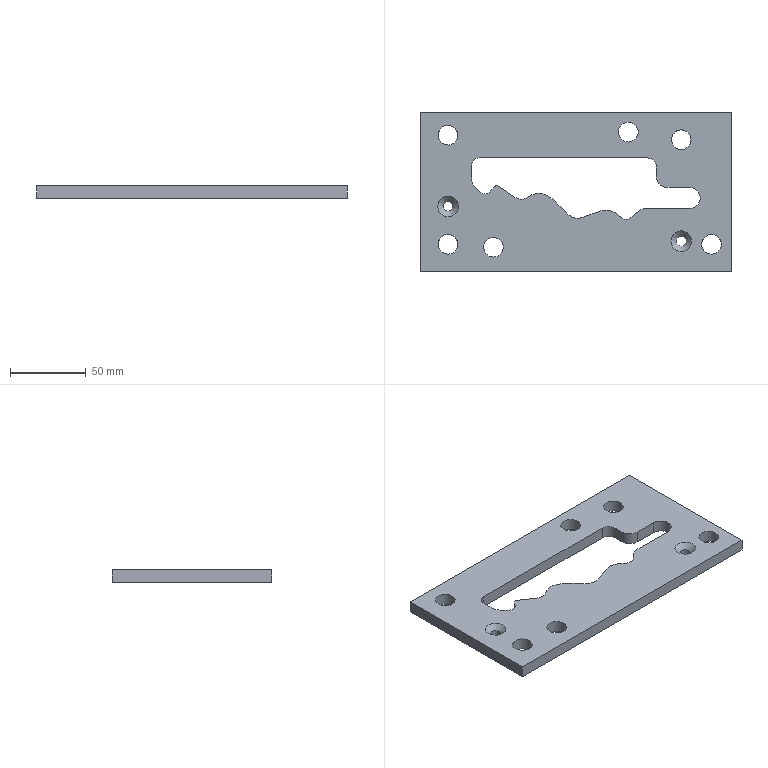Part | STEP file | gslz 2016.10.28-13_id754_x_t | 1 solid | 43 faces | box 205 x 105 x 8 mm | volume 132128 mm3 | cylinder 22 | plane 19 | cone 2 | commonest cylinder face diameters 13 x6 10 x3 14 x3 6.5 x2 16 x2 4 x1